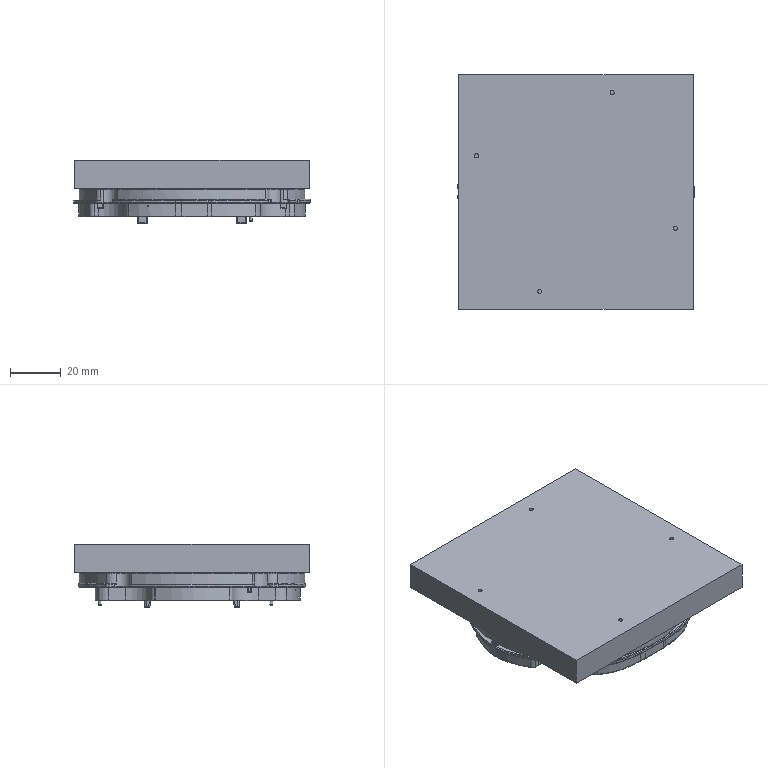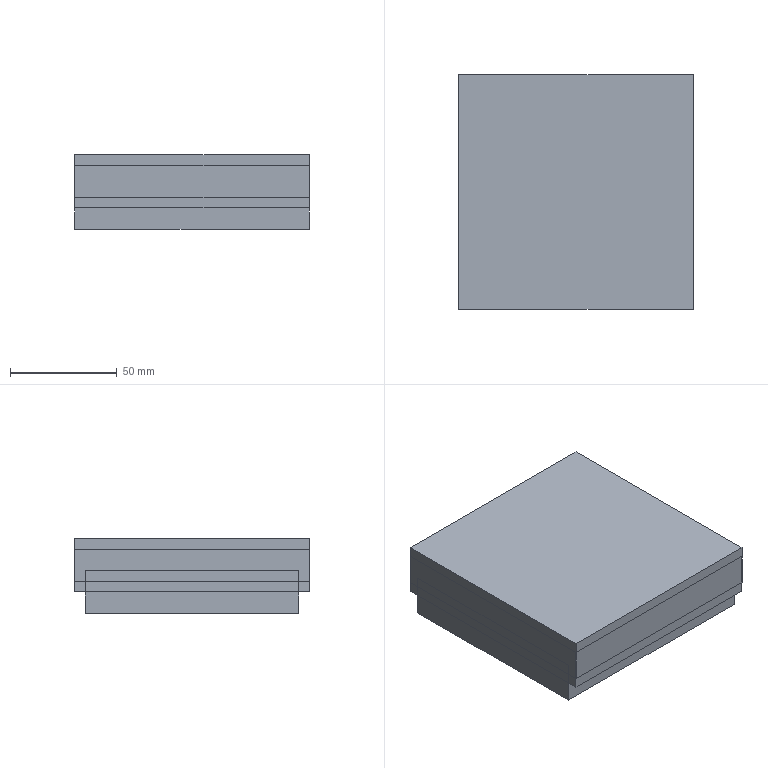CAM job | NX | 3-axis milling, drilling | part box 92.935 x 92.1 x 24.829 mm | stock box 110.034 x 110 x 34.947 mm
Tools:
number,name,description,diameter,corner_radius,flute_length,length,flutes
21,D1-10-D4-50-3T,D1*10*4*50-3T,1.0,0.0,10.0,11.0,3
19,D2-6-D4-50-3T-ROUGH,D2-6-D4-50-3T-粗,2.0,0.0,6.0,7.0,2
15,D3-9-D4-50-3T-ROUGH,D3-9-D4-50-3T,3.0,0.0,9.0,10.0,3
18,D3NEIR0.5,D3-9-D4-50-3T-精,3.0,0.0,9.0,10.0,2
12,D4-12-D4-50-3T-FINISH,D4-12-D4-50-3T,4.0,0.0,12.0,50.0,3
10,D8-25-D8-60-3T-ROUGH,D8-25-D8-60-3T-粗,8.0,0.0,25.0,60.0,2
16,D8-25-D8-60-3T-FINISH,D8-25-D8-60-3T,8.0,0.0,25.0,60.0,3
13,钻头D1.84-11-D3-40,钻刀D1.84-11-D3-40,1.84,0.0,11.0,12.0,2
12,钻头D2.5-35-61,钻刀D2.5-35-61,2.5,0.0,36.0,61.0,2
14,挤压M2-12-D3-39,挤压M2-12-D3-39,2.0,0.0,12.5,14.5,2
11,倒角D4-90度,倒角D4-90度,4.0,0.0,5.0,50.0,2
17,D3R0.2,Milling Tool-5 Parameters,3.0,0.2,50.0,75.0,2
0,R0.5,Milling Tool-5 Parameters,1.0,0.5,50.0,75.0,2
Operations:
program,operation,operation_type,tool,method,geometry_group,spindle_rpm,surface_speed,feed_per_tooth,feed_cut,feed_plunge,cut_length_mm,path_length_mm,cut_time_min,machine_time_min
A1,动态粗,CavityMilling,D8-25-D8-60-3T-ROUGH,METHOD,WORKPIECE_54,6500.0,100.0,0.1178,3000.0,100.0,13265.467,14220.783,4.257,4.353
A1,DRILLING,Operation,倒角D4-90度,METHOD,WORKPIECE_54,2500.0,31.0,0.04,200.0,0.0,32.0,367.907,0.16,0.1936
A1,DRILLING_1,Operation,钻头D2.5-35-61,METHOD,WORKPIECE_54,2500.0,19.0,0.04,200.0,0.0,52.0,337.953,0.26,0.2886
A1,DRILLING_2,Operation,钻头D1.84-11-D3-40,METHOD,WORKPIECE_54,1800.0,10.0,0.0333,120.0,0.0,34.4,296.099,0.2867,0.3128
A1,DRILLING_2_COPY,Operation,挤压M2-12-D3-39,METHOD,WORKPIECE_54,300.0,1.0,0.2,120.0,0.0,32.0,291.3,0.2667,0.2926
A1,PLANAR_MILL,PlanarMilling,D3-9-D4-50-3T-ROUGH,METHOD,WORKPIECE_54,3500.0,32.0,0.0762,800.0,100.0,2184.513,2311.61,2.731,2.743
A1,PLANAR_MILL_4,PlanarMilling,D3-9-D4-50-3T-ROUGH,METHOD,WORKPIECE_54,3500.0,32.0,0.1143,1200.0,100.0,387.448,712.764,0.3229,0.3554
A1,PLANAR_MILL_1,PlanarMilling,D3-9-D4-50-3T-ROUGH,METHOD,WORKPIECE_54,3500.0,32.0,0.0571,600.0,100.0,11.702,61.309,0.0195,0.0245
A1,PLANAR_MILL_1_COPY,PlanarMilling,D3-9-D4-50-3T-ROUGH,METHOD,WORKPIECE_54,3500.0,32.0,0.0571,600.0,100.0,99.158,460.429,0.1653,0.2014
A1,PLANAR_MILL_4_COPY,PlanarMilling,D3-9-D4-50-3T-ROUGH,METHOD,WORKPIECE_54,3500.0,32.0,0.0381,400.0,100.0,42.584,376.22,0.1065,0.1398
A1,PLANAR_MILL_2_COPY,PlanarMilling,D8-25-D8-60-3T-FINISH,METHOD,WORKPIECE_54,3500.0,87.0,0.0762,800.0,100.0,595.355,633.355,0.7442,0.748
A1,CAVITY_MILL,CavityMilling,D8-25-D8-60-3T-FINISH,METHOD,WORKPIECE_54,3500.0,87.0,0.0762,800.0,100.0,675.119,745.119,0.8439,0.8509
A1,PLANAR_MILL_2,PlanarMilling,D8-25-D8-60-3T-FINISH,METHOD,WORKPIECE_54,3500.0,87.0,0.0762,800.0,100.0,325.291,371.897,0.4066,0.4113
A1,PLANAR_MILL_2_COPY_1,PlanarMilling,D8-25-D8-60-3T-FINISH,METHOD,WORKPIECE_54,3500.0,87.0,0.0762,800.0,100.0,71.776,118.983,0.0897,0.0944
A1,FLOOR_FACING,VolumeBased25DMillingOperation,D8-25-D8-60-3T-FINISH,METHOD,WORKPIECE_54,3500.0,87.0,0.0762,800.0,100.0,819.692,862.798,1.025,1.029
A1,PLANAR_MILL_3,PlanarMilling,D3R0.2,METHOD,WORKPIECE_54,3500.0,43.0,0.0857,600.0,100.0,523.389,569.496,0.8723,0.8769
A1,PLANAR_MILL_13,PlanarMilling,D3NEIR0.5,METHOD,WORKPIECE_54,3500.0,32.0,0.0762,800.0,100.0,307.334,345.935,0.3842,0.388
A1,PLANAR_MILL_13_COPY,PlanarMilling,D3NEIR0.5,METHOD,WORKPIECE_54,3500.0,32.0,0.0762,800.0,100.0,261.438,300.038,0.3268,0.3307
A1,PLANAR_MILL_14,PlanarMilling,倒角D4-90度,METHOD,A-G54,3500.0,43.0,0.0429,300.0,100.0,50.436,361.645,0.1681,0.1992
A1,ZLEVEL_PROFILE_STEEP_1,ZLevelMilling,D3R0.2,METHOD,A-G54,4500.0,42.0,0.2222,2000.0,100.0,653.273,703.008,0.3266,0.3316
A1,ZLEVEL_PROFILE_STEEP_1_COPY,ZLevelMilling,D3R0.2,METHOD,A-G54,4500.0,42.0,0.2222,2000.0,100.0,3074.7,4414.62,1.537,1.671
A1,ZLEVEL_PROFILE_STEEP_2,ZLevelMilling,D1-10-D4-50-3T,METHOD,A-G54,4500.0,14.0,0.0444,600.0,100.0,200.645,250.797,0.3344,0.3394
B1,PLANAR_MILL_17,PlanarMilling,D8-25-D8-60-3T-ROUGH,METHOD,B-G55,4500.0,113.0,0.1333,1200.0,100.0,1068.049,1207.99,0.89,0.904
B1,PLANAR_MILL_17_COPY,PlanarMilling,D8-25-D8-60-3T-ROUGH,METHOD,B-G55,4500.0,113.0,0.1333,1200.0,100.0,1276.537,1418.654,1.064,1.078
B1,ADAPTIVE_MILLING,CavityMilling,D8-25-D8-60-3T-ROUGH,METHOD,WORKPIECE_55,5500.0,138.0,0.2727,3000.0,100.0,25603.486,29412.485,6.78,7.161
B1,ADAPTIVE_MILLING_COPY,CavityMilling,D3-9-D4-50-3T-ROUGH,METHOD,WORKPIECE_55,5500.0,138.0,0.2727,3000.0,100.0,4282.297,9630.146,1.253,1.788
B1,PLANAR_MILL_5,PlanarMilling,D2-6-D4-50-3T-ROUGH,METHOD,B-G55,4500.0,28.0,0.1333,1200.0,100.0,4424.545,8205.4,3.687,4.065
B1,PLANAR_MILL_6,PlanarMilling,D2-6-D4-50-3T-ROUGH,METHOD,B-G55,4500.0,28.0,0.1333,1200.0,100.0,434.717,675.497,0.3623,0.3863
B1,PLANAR_MILL_6_COPY,PlanarMilling,D2-6-D4-50-3T-ROUGH,METHOD,B-G55,4500.0,28.0,0.1333,1200.0,100.0,3778.983,6012.3,3.149,3.373
B1,PLANAR_MILL_7,PlanarMilling,D4-12-D4-50-3T-FINISH,METHOD,B-G55,4500.0,56.0,0.0593,800.0,100.0,1746.079,1792.13,2.183,2.187
B1,PLANAR_MILL_7_COPY_2,PlanarMilling,D4-12-D4-50-3T-FINISH,METHOD,B-G55,4500.0,56.0,0.0593,800.0,100.0,469.411,516.462,0.5868,0.5915
B1,PLANAR_MILL_7_COPY,PlanarMilling,D4-12-D4-50-3T-FINISH,METHOD,B-G55,4500.0,56.0,0.0593,800.0,100.0,438.947,489.198,0.5487,0.5537
B1,PLANAR_MILL_8,PlanarMilling,D4-12-D4-50-3T-FINISH,METHOD,B-G55,4500.0,56.0,0.0593,800.0,100.0,311.18,361.23,0.389,0.394
B1,PLANAR_MILL_8_COPY,PlanarMilling,D4-12-D4-50-3T-FINISH,METHOD,B-G55,4500.0,56.0,0.0593,800.0,100.0,60.589,232.53,0.0757,0.0929
B1,FLOOR_FACING_1,VolumeBased25DMillingOperation,D4-12-D4-50-3T-FINISH,METHOD,B-G55,4500.0,56.0,0.0593,800.0,100.0,436.01,1251.875,0.545,0.6266
B1,PLANAR_MILL_10,PlanarMilling,D4-12-D4-50-3T-FINISH,METHOD,B-G55,4500.0,56.0,0.0593,800.0,100.0,307.288,434.02,0.3841,0.3968
B1,FLOOR_FACING_1_COPY,VolumeBased25DMillingOperation,D4-12-D4-50-3T-FINISH,METHOD,B-G55,4500.0,56.0,0.0593,800.0,100.0,123.395,500.25,0.1542,0.1919
B1,FLOOR_FACING_1_COPY_COPY,VolumeBased25DMillingOperation,D4-12-D4-50-3T-FINISH,METHOD,B-G55,4500.0,56.0,0.0593,800.0,100.0,108.801,634.433,0.136,0.1886
B1,PLANAR_MILL_10_COPY,PlanarMilling,D4-12-D4-50-3T-FINISH,METHOD,B-G55,4500.0,56.0,0.0593,800.0,100.0,53.239,211.142,0.0665,0.0823
B1,PLANAR_MILL_11,PlanarMilling,D4-12-D4-50-3T-FINISH,METHOD,B-G55,4500.0,56.0,0.0593,800.0,100.0,20.037,64.288,0.025,0.0295
B1,PLANAR_MILL_11_COPY,PlanarMilling,D4-12-D4-50-3T-FINISH,METHOD,B-G55,4500.0,56.0,0.0593,800.0,100.0,31.477,129.506,0.0393,0.0491
B1,PLANAR_MILL_7_COPY_1,PlanarMilling,D3-9-D4-50-3T-ROUGH,METHOD,B-G55,4500.0,42.0,0.0444,600.0,100.0,281.257,327.308,0.4688,0.4734
B1,PLANAR_MILL_9,PlanarMilling,D3-9-D4-50-3T-ROUGH,METHOD,B-G55,4500.0,42.0,0.0444,600.0,100.0,574.908,614.759,0.9582,0.9622
B1,PLANAR_MILL_9_COPY,PlanarMilling,D3-9-D4-50-3T-ROUGH,METHOD,B-G55,4500.0,42.0,0.0444,600.0,100.0,324.032,374.683,0.5401,0.5451
B1,PLANAR_MILL_6_COPY_1,PlanarMilling,D1-10-D4-50-3T,METHOD,B-G55,4500.0,14.0,0.0444,600.0,100.0,908.08,1211.152,1.514,1.544
B1,PLANAR_MILL_6_COPY_COPY,PlanarMilling,D1-10-D4-50-3T,METHOD,B-G55,4500.0,14.0,0.0444,600.0,100.0,936.026,1452.82,1.56,1.612
B1,PLANAR_MILL_12,PlanarMilling,D1-10-D4-50-3T,METHOD,B-G55,4500.0,14.0,0.0444,600.0,100.0,2650.825,4708.199,4.418,4.624
B1,PLANAR_MILL_12_COPY,PlanarMilling,D1-10-D4-50-3T,METHOD,B-G55,4500.0,14.0,0.0444,600.0,100.0,777.434,1808.325,1.296,1.399
B1,ZLEVEL_PROFILE_STEEP,ZLevelMilling,D3R0.2,METHOD,B-G55,3500.0,43.0,0.2857,2000.0,100.0,10679.173,11152.33,5.34,5.387
B1,ZLEVEL_PROFILE_STEEP_COPY,ZLevelMilling,D3R0.2,METHOD,B-G55,3500.0,43.0,0.2857,2000.0,100.0,347.502,526.513,0.1738,0.1917
B1,CURVE_DRIVE,SurfaceContour,R0.5,METHOD,B-G55,4500.0,14.0,0.1111,1000.0,100.0,972.848,1022.998,0.9728,0.9779
B1,PLANAR_MILL_18,PlanarMilling,倒角D4-90度,METHOD,B-G55,3000.0,37.0,0.1,600.0,100.0,33.133,191.544,0.0552,0.0711
B1,DRILLING_3,Operation,倒角D4-90度,METHOD,B-G55,2000.0,25.0,0.05,200.0,0.0,15.2,259.072,0.076,0.1004
B1,DRILLING_3_COPY,Operation,钻头D1.84-11-D3-40,METHOD,B-G55,1600.0,9.0,0.0375,120.0,0.0,30.0,288.672,0.25,0.2759
B1,DRILLING_3_COPY_COPY,Operation,挤压M2-12-D3-39,METHOD,B-G55,300.0,1.0,0.2,120.0,0.0,28.0,284.672,0.2333,0.259
工装1,ADAPTIVE_MILLING_1,CavityMilling,D8-25-D8-60-3T-ROUGH,METHOD,WORKPIECE,5500.0,138.0,0.1818,2000.0,100.0,4134.124,4208.124,1.903,1.911
工装1,DRILLING_4,Operation,D8-25-D8-60-3T-ROUGH,METHOD,WORKPIECE,1600.0,40.0,0.0469,150.0,0.0,38.0,301.3,0.2533,0.2797
工装1,PLANAR_MILL_15,PlanarMilling,D8-25-D8-60-3T-FINISH,METHOD,WORKPIECE,4500.0,113.0,0.0593,800.0,100.0,403.816,469.816,0.5048,0.5114
工装2,ADAPTIVE_MILLING_2,CavityMilling,D8-25-D8-60-3T-ROUGH,METHOD,WORKPIECE_1,5500.0,138.0,0.2273,2500.0,100.0,15303.827,15903.448,5.297,5.357
工装2,FLOOR_FACING_2,VolumeBased25DMillingOperation,D8-25-D8-60-3T-FINISH,METHOD,GZ2,4500.0,113.0,0.0593,800.0,100.0,976.26,1076.261,1.22,1.23
工装2,ADAPTIVE_MILLING_2_COPY,CavityMilling,D3-9-D4-50-3T-ROUGH,METHOD,WORKPIECE_1,5500.0,51.0,0.0909,1500.0,100.0,511.85,1158.171,0.3017,0.3664
工装2,FLOOR_FACING_2_COPY,VolumeBased25DMillingOperation,D3-9-D4-50-3T-ROUGH,METHOD,GZ2,4500.0,42.0,0.0593,800.0,100.0,1975.657,2077.763,2.47,2.48
工装2,PLANAR_MILL_16,PlanarMilling,D3-9-D4-50-3T-ROUGH,METHOD,GZ2,4500.0,42.0,0.0593,800.0,100.0,61.579,338.983,0.077,0.1047
工装2,DRILLING_5,Operation,倒角D4-90度,METHOD,GZ2,2500.0,31.0,0.03,150.0,0.0,16.8,267.006,0.112,0.137
工装2,DRILLING_5_COPY,Operation,钻头D2.5-35-61,METHOD,GZ2,2500.0,31.0,0.03,150.0,0.0,52.0,337.406,0.3467,0.3752